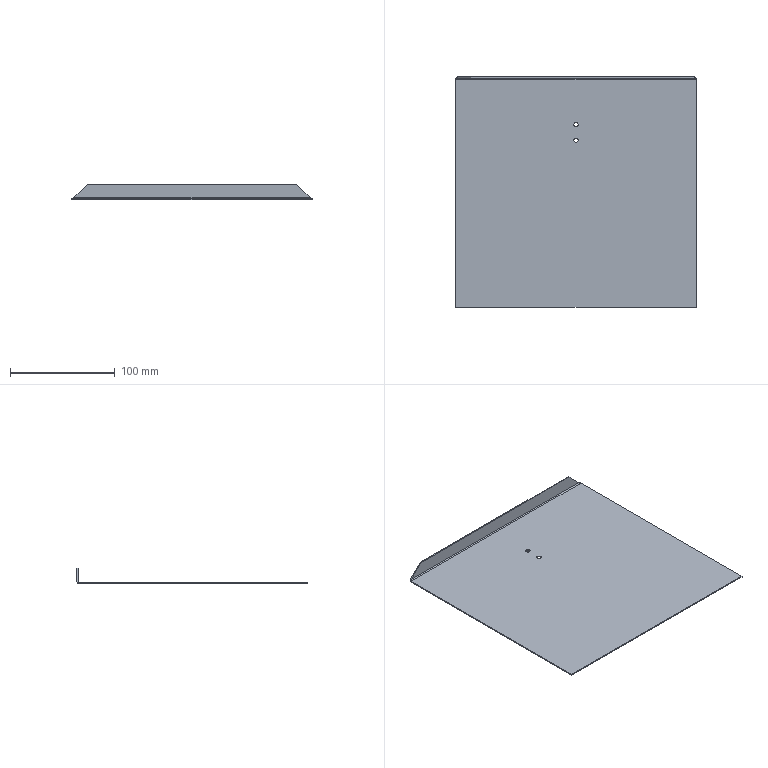Part | SolidWorks | features BaseBody 1 | 1 solid | 26 faces | box 230 x 220 x 15 mm | volume 53420 mm3 | plane 18 | cylinder 6 | spline 2 | commonest cylinder face diameters 4 x5 2 x1
STEP:
#1=CARTESIAN_POINT('',(113.,109.5,1.));
#2=VERTEX_POINT('',#1);
#3=CARTESIAN_POINT('',(113.,110.5,1.));
#4=VERTEX_POINT('',#3);
#5=CARTESIAN_POINT('',(113.,109.5,1.));
#6=DIRECTION('',(0.,1.,0.));
#7=VECTOR('',#6,1000.);
#8=LINE('',#5,#7);
#9=EDGE_CURVE('',#2,#4,#8,.T.);
#10=ORIENTED_EDGE('',*,*,#9,.F.);
#11=CARTESIAN_POINT('',(114.,108.5,0.));
#12=VERTEX_POINT('',#11);
#13=CARTESIAN_POINT('',(114.,108.5,0.));
#14=CARTESIAN_POINT('',(114.,109.086,0.));
#15=CARTESIAN_POINT('',(113.586,109.5,0.4142));
#16=CARTESIAN_POINT('',(113.,109.5,1.));
#17=(BOUNDED_CURVE()B_SPLINE_CURVE(3,(#13,#14,#15,#16),.UNSPECIFIED.,.F.,.F.)B_SPLINE_CURVE_WITH_KNOTS((4,4),(3.142,4.712),.UNSPECIFIED.)CURVE()GEOMETRIC_REPRESENTATION_ITEM()RATIONAL_B_SPLINE_CURVE((1.,0.8047,0.8047,1.))REPRESENTATION_ITEM(''));
#18=EDGE_CURVE('',#12,#2,#17,.T.);
#19=ORIENTED_EDGE('',*,*,#18,.F.);
#20=CARTESIAN_POINT('',(114.,108.5,-1.));
#21=VERTEX_POINT('',#20);
#22=CARTESIAN_POINT('',(114.,108.5,0.));
#23=DIRECTION('',(0.,0.,-1.));
#24=VECTOR('',#23,1000.);
#25=LINE('',#22,#24);
#26=EDGE_CURVE('',#12,#21,#25,.T.);
#27=ORIENTED_EDGE('',*,*,#26,.T.);
#28=CARTESIAN_POINT('',(114.,108.5,-1.));
#29=CARTESIAN_POINT('',(114.,109.672,-1.));
#30=CARTESIAN_POINT('',(113.586,110.5,-0.1716));
#31=CARTESIAN_POINT('',(113.,110.5,1.));
#32=(BOUNDED_CURVE()B_SPLINE_CURVE(3,(#28,#29,#30,#31),.UNSPECIFIED.,.F.,.F.)B_SPLINE_CURVE_WITH_KNOTS((4,4),(3.142,4.712),.UNSPECIFIED.)CURVE()GEOMETRIC_REPRESENTATION_ITEM()RATIONAL_B_SPLINE_CURVE((1.,0.8047,0.8047,1.))REPRESENTATION_ITEM(''));
#33=EDGE_CURVE('',#21,#4,#32,.T.);
#34=ORIENTED_EDGE('',*,*,#33,.T.);
#35=EDGE_LOOP('',(#10,#19,#27,#34));
#36=FACE_OUTER_BOUND('',#35,.T.);
#37=CARTESIAN_POINT('',(114.,108.5,-1.));
#38=CARTESIAN_POINT('',(114.,108.5,-0.6667));
#39=CARTESIAN_POINT('',(114.,108.5,-0.3333));
#40=CARTESIAN_POINT('',(114.,108.5,0.));
#41=CARTESIAN_POINT('',(114.,109.5,-1.));
#42=CARTESIAN_POINT('',(114.,109.333,-0.6667));
#43=CARTESIAN_POINT('',(114.,109.167,-0.3333));
#44=CARTESIAN_POINT('',(114.,109.,0.));
#45=CARTESIAN_POINT('',(113.667,110.5,-0.3333));
#46=CARTESIAN_POINT('',(113.667,110.167,-0.1111));
#47=CARTESIAN_POINT('',(113.667,109.833,0.1111));
#48=CARTESIAN_POINT('',(113.667,109.5,0.3333));
#49=CARTESIAN_POINT('',(113.,110.5,1.));
#50=CARTESIAN_POINT('',(113.,110.167,1.));
#51=CARTESIAN_POINT('',(113.,109.833,1.));
#52=CARTESIAN_POINT('',(113.,109.5,1.));
#53=(BOUNDED_SURFACE()B_SPLINE_SURFACE(3,3,((#37,#38,#39,#40),(#41,#42,#43,#44),(#45,#46,#47,#48),(#49,#50,#51,#52)),.UNSPECIFIED.,.F.,.F.,.T.)B_SPLINE_SURFACE_WITH_KNOTS((4,4),(4,4),(0.5,0.75),(0.,1.),.UNSPECIFIED.)GEOMETRIC_REPRESENTATION_ITEM()RATIONAL_B_SPLINE_SURFACE(((1.,1.,1.,1.),(0.6667,0.6667,0.6667,0.6667),(0.5,0.5,0.5,0.5),(0.5,0.5,0.5,0.5)))REPRESENTATION_ITEM('')SURFACE());
#54=ADVANCED_FACE('',(#36),#53,.T.);
#55=CARTESIAN_POINT('',(100.,109.5,14.));
#56=VERTEX_POINT('',#55);
#57=CARTESIAN_POINT('',(57.,109.5,57.));
#58=DIRECTION('',(0.7071,0.,-0.7071));
#59=VECTOR('',#58,1000.);
#60=LINE('',#57,#59);
#61=EDGE_CURVE('',#56,#2,#60,.T.);
#62=ORIENTED_EDGE('',*,*,#61,.T.);
#63=ORIENTED_EDGE('',*,*,#9,.T.);
#64=CARTESIAN_POINT('',(100.,110.5,14.));
#65=VERTEX_POINT('',#64);
#66=CARTESIAN_POINT('',(57.,110.5,57.));
#67=DIRECTION('',(0.7071,0.,-0.7071));
#68=VECTOR('',#67,1000.);
#69=LINE('',#66,#68);
#70=EDGE_CURVE('',#65,#4,#69,.T.);
#71=ORIENTED_EDGE('',*,*,#70,.F.);
#72=CARTESIAN_POINT('',(100.,109.5,14.));
#73=DIRECTION('',(0.,1.,0.));
#74=VECTOR('',#73,1000.);
#75=LINE('',#72,#74);
#76=EDGE_CURVE('',#56,#65,#75,.T.);
#77=ORIENTED_EDGE('',*,*,#76,.F.);
#78=EDGE_LOOP('',(#62,#63,#71,#77));
#79=FACE_OUTER_BOUND('',#78,.T.);
#80=CARTESIAN_POINT('',(57.,109.5,57.));
#81=DIRECTION('',(-0.7071,0.,-0.7071));
#82=DIRECTION('',(-0.7071,0.,0.7071));
#83=AXIS2_PLACEMENT_3D('',#80,#81,#82);
#84=PLANE('',#83);
#85=ADVANCED_FACE('',(#79),#84,.F.);
#86=CARTESIAN_POINT('',(-114.,108.5,0.));
#87=VERTEX_POINT('',#86);
#88=CARTESIAN_POINT('',(-114.,108.5,-1.));
#89=VERTEX_POINT('',#88);
#90=CARTESIAN_POINT('',(-114.,108.5,0.));
#91=DIRECTION('',(0.,0.,-1.));
#92=VECTOR('',#91,1000.);
#93=LINE('',#90,#92);
#94=EDGE_CURVE('',#87,#89,#93,.T.);
#95=ORIENTED_EDGE('',*,*,#94,.F.);
#96=CARTESIAN_POINT('',(-113.,109.5,1.));
#97=VERTEX_POINT('',#96);
#98=CARTESIAN_POINT('',(-113.,109.5,1.));
#99=CARTESIAN_POINT('',(-113.586,109.5,0.4142));
#100=CARTESIAN_POINT('',(-114.,109.086,0.));
#101=CARTESIAN_POINT('',(-114.,108.5,0.));
#102=(BOUNDED_CURVE()B_SPLINE_CURVE(3,(#98,#99,#100,#101),.UNSPECIFIED.,.F.,.F.)B_SPLINE_CURVE_WITH_KNOTS((4,4),(4.712,6.283),.UNSPECIFIED.)CURVE()GEOMETRIC_REPRESENTATION_ITEM()RATIONAL_B_SPLINE_CURVE((1.,0.8047,0.8047,1.))REPRESENTATION_ITEM(''));
#103=EDGE_CURVE('',#97,#87,#102,.T.);
#104=ORIENTED_EDGE('',*,*,#103,.F.);
#105=CARTESIAN_POINT('',(-113.,110.5,1.));
#106=VERTEX_POINT('',#105);
#107=CARTESIAN_POINT('',(-113.,110.5,1.));
#108=DIRECTION('',(0.,-1.,0.));
#109=VECTOR('',#108,1000.);
#110=LINE('',#107,#109);
#111=EDGE_CURVE('',#106,#97,#110,.T.);
#112=ORIENTED_EDGE('',*,*,#111,.F.);
#113=CARTESIAN_POINT('',(-113.,110.5,1.));
#114=CARTESIAN_POINT('',(-113.586,110.5,-0.1716));
#115=CARTESIAN_POINT('',(-114.,109.672,-1.));
#116=CARTESIAN_POINT('',(-114.,108.5,-1.));
#117=(BOUNDED_CURVE()B_SPLINE_CURVE(3,(#113,#114,#115,#116),.UNSPECIFIED.,.F.,.F.)B_SPLINE_CURVE_WITH_KNOTS((4,4),(4.712,6.283),.UNSPECIFIED.)CURVE()GEOMETRIC_REPRESENTATION_ITEM()RATIONAL_B_SPLINE_CURVE((1.,0.8047,0.8047,1.))REPRESENTATION_ITEM(''));
#118=EDGE_CURVE('',#106,#89,#117,.T.);
#119=ORIENTED_EDGE('',*,*,#118,.T.);
#120=EDGE_LOOP('',(#95,#104,#112,#119));
#121=FACE_OUTER_BOUND('',#120,.T.);
#122=CARTESIAN_POINT('',(-113.,110.5,1.));
#123=CARTESIAN_POINT('',(-113.,110.167,1.));
#124=CARTESIAN_POINT('',(-113.,109.833,1.));
#125=CARTESIAN_POINT('',(-113.,109.5,1.));
#126=CARTESIAN_POINT('',(-113.667,110.5,-0.3333));
#127=CARTESIAN_POINT('',(-113.667,110.167,-0.1111));
#128=CARTESIAN_POINT('',(-113.667,109.833,0.1111));
#129=CARTESIAN_POINT('',(-113.667,109.5,0.3333));
#130=CARTESIAN_POINT('',(-114.,109.5,-1.));
#131=CARTESIAN_POINT('',(-114.,109.333,-0.6667));
#132=CARTESIAN_POINT('',(-114.,109.167,-0.3333));
#133=CARTESIAN_POINT('',(-114.,109.,0.));
#134=CARTESIAN_POINT('',(-114.,108.5,-1.));
#135=CARTESIAN_POINT('',(-114.,108.5,-0.6667));
#136=CARTESIAN_POINT('',(-114.,108.5,-0.3333));
#137=CARTESIAN_POINT('',(-114.,108.5,0.));
#138=(BOUNDED_SURFACE()B_SPLINE_SURFACE(3,3,((#122,#123,#124,#125),(#126,#127,#128,#129),(#130,#131,#132,#133),(#134,#135,#136,#137)),.UNSPECIFIED.,.F.,.F.,.T.)B_SPLINE_SURFACE_WITH_KNOTS((4,4),(4,4),(0.75,1.),(0.,1.),.UNSPECIFIED.)GEOMETRIC_REPRESENTATION_ITEM()RATIONAL_B_SPLINE_SURFACE(((0.5,0.5,0.5,0.5),(0.5,0.5,0.5,0.5),(0.6667,0.6667,0.6667,0.6667),(1.,1.,1.,1.)))REPRESENTATION_ITEM('')SURFACE());
#139=ADVANCED_FACE('',(#121),#138,.T.);
#140=CARTESIAN_POINT('',(-100.,110.5,14.));
#141=VERTEX_POINT('',#140);
#142=CARTESIAN_POINT('',(-100.,109.5,14.));
#143=VERTEX_POINT('',#142);
#144=CARTESIAN_POINT('',(-100.,110.5,14.));
#145=DIRECTION('',(0.,-1.,0.));
#146=VECTOR('',#145,1000.);
#147=LINE('',#144,#146);
#148=EDGE_CURVE('',#141,#143,#147,.T.);
#149=ORIENTED_EDGE('',*,*,#148,.F.);
#150=CARTESIAN_POINT('',(-114.,110.5,0.));
#151=DIRECTION('',(-0.7071,0.,-0.7071));
#152=VECTOR('',#151,1000.);
#153=LINE('',#150,#152);
#154=EDGE_CURVE('',#141,#106,#153,.T.);
#155=ORIENTED_EDGE('',*,*,#154,.T.);
#156=ORIENTED_EDGE('',*,*,#111,.T.);
#157=CARTESIAN_POINT('',(-114.,109.5,0.));
#158=DIRECTION('',(-0.7071,0.,-0.7071));
#159=VECTOR('',#158,1000.);
#160=LINE('',#157,#159);
#161=EDGE_CURVE('',#143,#97,#160,.T.);
#162=ORIENTED_EDGE('',*,*,#161,.F.);
#163=EDGE_LOOP('',(#149,#155,#156,#162));
#164=FACE_OUTER_BOUND('',#163,.T.);
#165=CARTESIAN_POINT('',(-114.,110.5,0.));
#166=DIRECTION('',(-0.7071,0.,0.7071));
#167=DIRECTION('',(0.,1.,0.));
#168=AXIS2_PLACEMENT_3D('',#165,#166,#167);
#169=PLANE('',#168);
#170=ADVANCED_FACE('',(#164),#169,.T.);
#171=CARTESIAN_POINT('',(114.5,109.5,0.));
#172=VERTEX_POINT('',#171);
#173=CARTESIAN_POINT('',(114.5,109.5,-1.));
#174=VERTEX_POINT('',#173);
#175=CARTESIAN_POINT('',(114.5,109.5,0.));
#176=DIRECTION('',(0.,0.,-1.));
#177=VECTOR('',#176,1000.);
#178=LINE('',#175,#177);
#179=EDGE_CURVE('',#172,#174,#178,.T.);
#180=ORIENTED_EDGE('',*,*,#179,.T.);
#181=CARTESIAN_POINT('',(114.5,108.,-1.));
#182=VERTEX_POINT('',#181);
#183=CARTESIAN_POINT('',(114.5,-109.5,-1.));
#184=DIRECTION('',(0.,-1.,0.));
#185=VECTOR('',#184,1000.);
#186=LINE('',#183,#185);
#187=EDGE_CURVE('',#174,#182,#186,.T.);
#188=ORIENTED_EDGE('',*,*,#187,.T.);
#189=CARTESIAN_POINT('',(114.5,108.,0.));
#190=VERTEX_POINT('',#189);
#191=CARTESIAN_POINT('',(114.5,108.,0.));
#192=DIRECTION('',(0.,0.,-1.));
#193=VECTOR('',#192,1000.);
#194=LINE('',#191,#193);
#195=EDGE_CURVE('',#190,#182,#194,.T.);
#196=ORIENTED_EDGE('',*,*,#195,.F.);
#197=CARTESIAN_POINT('',(114.5,108.,0.));
#198=DIRECTION('',(0.,1.,0.));
#199=VECTOR('',#198,1000.);
#200=LINE('',#197,#199);
#201=EDGE_CURVE('',#190,#172,#200,.T.);
#202=ORIENTED_EDGE('',*,*,#201,.T.);
#203=EDGE_LOOP('',(#180,#188,#196,#202));
#204=FACE_OUTER_BOUND('',#203,.T.);
#205=CARTESIAN_POINT('',(114.5,108.,0.));
#206=DIRECTION('',(-1.,0.,0.));
#207=DIRECTION('',(0.,1.,0.));
#208=AXIS2_PLACEMENT_3D('',#205,#206,#207);
#209=PLANE('',#208);
#210=ADVANCED_FACE('',(#204),#209,.T.);
#211=ORIENTED_EDGE('',*,*,#195,.T.);
#212=CARTESIAN_POINT('',(114.,108.,-1.));
#213=VERTEX_POINT('',#212);
#214=CARTESIAN_POINT('',(115.,108.,-1.));
#215=DIRECTION('',(-1.,0.,0.));
#216=VECTOR('',#215,1000.);
#217=LINE('',#214,#216);
#218=EDGE_CURVE('',#182,#213,#217,.T.);
#219=ORIENTED_EDGE('',*,*,#218,.T.);
#220=CARTESIAN_POINT('',(114.,108.,0.));
#221=VERTEX_POINT('',#220);
#222=CARTESIAN_POINT('',(114.,108.,0.));
#223=DIRECTION('',(0.,0.,-1.));
#224=VECTOR('',#223,1000.);
#225=LINE('',#222,#224);
#226=EDGE_CURVE('',#221,#213,#225,.T.);
#227=ORIENTED_EDGE('',*,*,#226,.F.);
#228=CARTESIAN_POINT('',(114.,108.,0.));
#229=DIRECTION('',(1.,0.,0.));
#230=VECTOR('',#229,1000.);
#231=LINE('',#228,#230);
#232=EDGE_CURVE('',#221,#190,#231,.T.);
#233=ORIENTED_EDGE('',*,*,#232,.T.);
#234=EDGE_LOOP('',(#211,#219,#227,#233));
#235=FACE_OUTER_BOUND('',#234,.T.);
#236=CARTESIAN_POINT('',(114.,108.,0.));
#237=DIRECTION('',(0.,1.,0.));
#238=DIRECTION('',(0.,0.,-1.));
#239=AXIS2_PLACEMENT_3D('',#236,#237,#238);
#240=PLANE('',#239);
#241=ADVANCED_FACE('',(#235),#240,.T.);
#242=ORIENTED_EDGE('',*,*,#226,.T.);
#243=CARTESIAN_POINT('',(114.,-109.5,-1.));
#244=DIRECTION('',(0.,1.,0.));
#245=VECTOR('',#244,1000.);
#246=LINE('',#243,#245);
#247=EDGE_CURVE('',#213,#21,#246,.T.);
#248=ORIENTED_EDGE('',*,*,#247,.T.);
#249=ORIENTED_EDGE('',*,*,#26,.F.);
#250=CARTESIAN_POINT('',(114.,108.5,0.));
#251=DIRECTION('',(0.,-1.,0.));
#252=VECTOR('',#251,1000.);
#253=LINE('',#250,#252);
#254=EDGE_CURVE('',#12,#221,#253,.T.);
#255=ORIENTED_EDGE('',*,*,#254,.T.);
#256=EDGE_LOOP('',(#242,#248,#249,#255));
#257=FACE_OUTER_BOUND('',#256,.T.);
#258=CARTESIAN_POINT('',(114.,108.5,0.));
#259=DIRECTION('',(1.,0.,0.));
#260=DIRECTION('',(0.,1.,0.));
#261=AXIS2_PLACEMENT_3D('',#258,#259,#260);
#262=PLANE('',#261);
#263=ADVANCED_FACE('',(#257),#262,.T.);
#264=ORIENTED_EDGE('',*,*,#94,.T.);
#265=CARTESIAN_POINT('',(-114.,108.,-1.));
#266=VERTEX_POINT('',#265);
#267=CARTESIAN_POINT('',(-114.,-109.5,-1.));
#268=DIRECTION('',(0.,-1.,0.));
#269=VECTOR('',#268,1000.);
#270=LINE('',#267,#269);
#271=EDGE_CURVE('',#89,#266,#270,.T.);
#272=ORIENTED_EDGE('',*,*,#271,.T.);
#273=CARTESIAN_POINT('',(-114.,108.,0.));
#274=VERTEX_POINT('',#273);
#275=CARTESIAN_POINT('',(-114.,108.,0.));
#276=DIRECTION('',(0.,0.,-1.));
#277=VECTOR('',#276,1000.);
#278=LINE('',#275,#277);
#279=EDGE_CURVE('',#274,#266,#278,.T.);
#280=ORIENTED_EDGE('',*,*,#279,.F.);
#281=CARTESIAN_POINT('',(-114.,108.,0.));
#282=DIRECTION('',(0.,1.,0.));
#283=VECTOR('',#282,1000.);
#284=LINE('',#281,#283);
#285=EDGE_CURVE('',#274,#87,#284,.T.);
#286=ORIENTED_EDGE('',*,*,#285,.T.);
#287=EDGE_LOOP('',(#264,#272,#280,#286));
#288=FACE_OUTER_BOUND('',#287,.T.);
#289=CARTESIAN_POINT('',(-114.,108.,0.));
#290=DIRECTION('',(-1.,0.,0.));
#291=DIRECTION('',(0.,0.,1.));
#292=AXIS2_PLACEMENT_3D('',#289,#290,#291);
#293=PLANE('',#292);
#294=ADVANCED_FACE('',(#288),#293,.T.);
#295=ORIENTED_EDGE('',*,*,#279,.T.);
#296=CARTESIAN_POINT('',(-114.5,108.,-1.));
#297=VERTEX_POINT('',#296);
#298=CARTESIAN_POINT('',(115.,108.,-1.));
#299=DIRECTION('',(-1.,0.,0.));
#300=VECTOR('',#299,1000.);
#301=LINE('',#298,#300);
#302=EDGE_CURVE('',#266,#297,#301,.T.);
#303=ORIENTED_EDGE('',*,*,#302,.T.);
#304=CARTESIAN_POINT('',(-114.5,108.,0.));
#305=VERTEX_POINT('',#304);
#306=CARTESIAN_POINT('',(-114.5,108.,0.));
#307=DIRECTION('',(0.,0.,-1.));
#308=VECTOR('',#307,1000.);
#309=LINE('',#306,#308);
#310=EDGE_CURVE('',#305,#297,#309,.T.);
#311=ORIENTED_EDGE('',*,*,#310,.F.);
#312=CARTESIAN_POINT('',(-114.5,108.,0.));
#313=DIRECTION('',(1.,0.,0.));
#314=VECTOR('',#313,1000.);
#315=LINE('',#312,#314);
#316=EDGE_CURVE('',#305,#274,#315,.T.);
#317=ORIENTED_EDGE('',*,*,#316,.T.);
#318=EDGE_LOOP('',(#295,#303,#311,#317));
#319=FACE_OUTER_BOUND('',#318,.T.);
#320=CARTESIAN_POINT('',(-114.5,108.,0.));
#321=DIRECTION('',(0.,1.,0.));
#322=DIRECTION('',(0.,0.,-1.));
#323=AXIS2_PLACEMENT_3D('',#320,#321,#322);
#324=PLANE('',#323);
#325=ADVANCED_FACE('',(#319),#324,.T.);
#326=ORIENTED_EDGE('',*,*,#310,.T.);
#327=CARTESIAN_POINT('',(-114.5,109.5,-1.));
#328=VERTEX_POINT('',#327);
#329=CARTESIAN_POINT('',(-114.5,-109.5,-1.));
#330=DIRECTION('',(0.,1.,0.));
#331=VECTOR('',#330,1000.);
#332=LINE('',#329,#331);
#333=EDGE_CURVE('',#297,#328,#332,.T.);
#334=ORIENTED_EDGE('',*,*,#333,.T.);
#335=CARTESIAN_POINT('',(-114.5,109.5,0.));
#336=VERTEX_POINT('',#335);
#337=CARTESIAN_POINT('',(-114.5,109.5,0.));
#338=DIRECTION('',(0.,0.,-1.));
#339=VECTOR('',#338,1000.);
#340=LINE('',#337,#339);
#341=EDGE_CURVE('',#336,#328,#340,.T.);
#342=ORIENTED_EDGE('',*,*,#341,.F.);
#343=CARTESIAN_POINT('',(-114.5,109.5,0.));
#344=DIRECTION('',(0.,-1.,0.));
#345=VECTOR('',#344,1000.);
#346=LINE('',#343,#345);
#347=EDGE_CURVE('',#336,#305,#346,.T.);
#348=ORIENTED_EDGE('',*,*,#347,.T.);
#349=EDGE_LOOP('',(#326,#334,#342,#348));
#350=FACE_OUTER_BOUND('',#349,.T.);
#351=CARTESIAN_POINT('',(-114.5,109.5,0.));
#352=DIRECTION('',(1.,0.,0.));
#353=DIRECTION('',(0.,1.,0.));
#354=AXIS2_PLACEMENT_3D('',#351,#352,#353);
#355=PLANE('',#354);
#356=ADVANCED_FACE('',(#350),#355,.T.);
#357=CARTESIAN_POINT('',(2.,65.,0.));
#358=VERTEX_POINT('',#357);
#359=CARTESIAN_POINT('',(2.,65.,-1.));
#360=VERTEX_POINT('',#359);
#361=CARTESIAN_POINT('',(2.,65.,9.));
#362=DIRECTION('',(0.,0.,-1.));
#363=VECTOR('',#362,1000.);
#364=LINE('',#361,#363);
#365=EDGE_CURVE('',#358,#360,#364,.T.);
#366=ORIENTED_EDGE('',*,*,#365,.F.);
#367=CARTESIAN_POINT('',(-2.,65.,0.));
#368=VERTEX_POINT('',#367);
#369=CARTESIAN_POINT('',(0.,65.,0.));
#370=DIRECTION('',(0.,0.,1.));
#371=DIRECTION('',(1.,0.,0.));
#372=AXIS2_PLACEMENT_3D('',#369,#370,#371);
#373=CIRCLE('',#372,2.);
#374=EDGE_CURVE('',#358,#368,#373,.T.);
#375=ORIENTED_EDGE('',*,*,#374,.T.);
#376=CARTESIAN_POINT('',(-2.,65.,-1.));
#377=VERTEX_POINT('',#376);
#378=CARTESIAN_POINT('',(-2.,65.,9.));
#379=DIRECTION('',(0.,0.,-1.));
#380=VECTOR('',#379,1000.);
#381=LINE('',#378,#380);
#382=EDGE_CURVE('',#368,#377,#381,.T.);
#383=ORIENTED_EDGE('',*,*,#382,.T.);
#384=CARTESIAN_POINT('',(0.,65.,-1.));
#385=DIRECTION('',(0.,0.,-1.));
#386=DIRECTION('',(-1.,0.,0.));
#387=AXIS2_PLACEMENT_3D('',#384,#385,#386);
#388=CIRCLE('',#387,2.);
#389=EDGE_CURVE('',#377,#360,#388,.T.);
#390=ORIENTED_EDGE('',*,*,#389,.T.);
#391=EDGE_LOOP('',(#366,#375,#383,#390));
#392=FACE_OUTER_BOUND('',#391,.T.);
#393=CARTESIAN_POINT('',(0.,65.,9.));
#394=DIRECTION('',(0.,0.,-1.));
#395=DIRECTION('',(-1.,0.,0.));
#396=AXIS2_PLACEMENT_3D('',#393,#394,#395);
#397=CYLINDRICAL_SURFACE('',#396,2.);
#398=ADVANCED_FACE('',(#392),#397,.F.);
#399=CARTESIAN_POINT('',(2.,50.,0.));
#400=VERTEX_POINT('',#399);
#401=CARTESIAN_POINT('',(2.,50.,-1.));
#402=VERTEX_POINT('',#401);
#403=CARTESIAN_POINT('',(2.,50.,9.));
#404=DIRECTION('',(0.,0.,-1.));
#405=VECTOR('',#404,1000.);
#406=LINE('',#403,#405);
#407=EDGE_CURVE('',#400,#402,#406,.T.);
#408=ORIENTED_EDGE('',*,*,#407,.F.);
#409=CARTESIAN_POINT('',(-2.,50.,0.));
#410=VERTEX_POINT('',#409);
#411=CARTESIAN_POINT('',(0.,50.,0.));
#412=DIRECTION('',(0.,0.,1.));
#413=DIRECTION('',(1.,0.,0.));
#414=AXIS2_PLACEMENT_3D('',#411,#412,#413);
#415=CIRCLE('',#414,2.);
#416=EDGE_CURVE('',#400,#410,#415,.T.);
#417=ORIENTED_EDGE('',*,*,#416,.T.);
#418=CARTESIAN_POINT('',(-2.,50.,-1.));
#419=VERTEX_POINT('',#418);
#420=CARTESIAN_POINT('',(-2.,50.,9.));
#421=DIRECTION('',(0.,0.,-1.));
#422=VECTOR('',#421,1000.);
#423=LINE('',#420,#422);
#424=EDGE_CURVE('',#410,#419,#423,.T.);
#425=ORIENTED_EDGE('',*,*,#424,.T.);
#426=CARTESIAN_POINT('',(0.,50.,-1.));
#427=DIRECTION('',(0.,0.,-1.));
#428=DIRECTION('',(-1.,0.,0.));
#429=AXIS2_PLACEMENT_3D('',#426,#427,#428);
#430=CIRCLE('',#429,2.);
#431=EDGE_CURVE('',#419,#402,#430,.T.);
#432=ORIENTED_EDGE('',*,*,#431,.T.);
#433=EDGE_LOOP('',(#408,#417,#425,#432));
#434=FACE_OUTER_BOUND('',#433,.T.);
#435=CARTESIAN_POINT('',(0.,50.,9.));
#436=DIRECTION('',(0.,0.,-1.));
#437=DIRECTION('',(-1.,0.,0.));
#438=AXIS2_PLACEMENT_3D('',#435,#436,#437);
#439=CYLINDRICAL_SURFACE('',#438,2.);
#440=ADVANCED_FACE('',(#434),#439,.F.);
#441=CARTESIAN_POINT('',(-115.,109.5,0.));
#442=VERTEX_POINT('',#441);
#443=CARTESIAN_POINT('',(-115.,-109.5,0.));
#444=VERTEX_POINT('',#443);
#445=CARTESIAN_POINT('',(-115.,109.5,0.));
#446=DIRECTION('',(0.,-1.,0.));
#447=VECTOR('',#446,1000.);
#448=LINE('',#445,#447);
#449=EDGE_CURVE('',#442,#444,#448,.T.);
#450=ORIENTED_EDGE('',*,*,#449,.F.);
#451=CARTESIAN_POINT('',(-115.,109.5,-1.));
#452=VERTEX_POINT('',#451);
#453=CARTESIAN_POINT('',(-115.,109.5,-1.));
#454=DIRECTION('',(0.,0.,1.));
#455=VECTOR('',#454,1000.);
#456=LINE('',#453,#455);
#457=EDGE_CURVE('',#452,#442,#456,.T.);
#458=ORIENTED_EDGE('',*,*,#457,.F.);
#459=CARTESIAN_POINT('',(-115.,-109.5,-1.));
#460=VERTEX_POINT('',#459);
#461=CARTESIAN_POINT('',(-115.,109.5,-1.));
#462=DIRECTION('',(0.,-1.,0.));
#463=VECTOR('',#462,1000.);
#464=LINE('',#461,#463);
#465=EDGE_CURVE('',#452,#460,#464,.T.);
#466=ORIENTED_EDGE('',*,*,#465,.T.);
#467=CARTESIAN_POINT('',(-115.,-109.5,-1.));
#468=DIRECTION('',(0.,0.,1.));
#469=VECTOR('',#468,1000.);
#470=LINE('',#467,#469);
#471=EDGE_CURVE('',#460,#444,#470,.T.);
#472=ORIENTED_EDGE('',*,*,#471,.T.);
#473=EDGE_LOOP('',(#450,#458,#466,#472));
#474=FACE_OUTER_BOUND('',#473,.T.);
#475=CARTESIAN_POINT('',(-115.,109.5,-1.));
#476=DIRECTION('',(-1.,0.,0.));
#477=DIRECTION('',(0.,1.,0.));
#478=AXIS2_PLACEMENT_3D('',#475,#476,#477);
#479=PLANE('',#478);
#480=ADVANCED_FACE('',(#474),#479,.T.);
#481=CARTESIAN_POINT('',(115.,-109.5,0.));
#482=VERTEX_POINT('',#481);
#483=CARTESIAN_POINT('',(-115.,-109.5,0.));
#484=DIRECTION('',(1.,0.,0.));
#485=VECTOR('',#484,1000.);
#486=LINE('',#483,#485);
#487=EDGE_CURVE('',#444,#482,#486,.T.);
#488=ORIENTED_EDGE('',*,*,#487,.F.);
#489=ORIENTED_EDGE('',*,*,#471,.F.);
#490=CARTESIAN_POINT('',(115.,-109.5,-1.));
#491=VERTEX_POINT('',#490);
#492=CARTESIAN_POINT('',(-115.,-109.5,-1.));
#493=DIRECTION('',(1.,0.,0.));
#494=VECTOR('',#493,1000.);
#495=LINE('',#492,#494);
#496=EDGE_CURVE('',#460,#491,#495,.T.);
#497=ORIENTED_EDGE('',*,*,#496,.T.);
#498=CARTESIAN_POINT('',(115.,-109.5,-1.));
#499=DIRECTION('',(0.,0.,1.));
#500=VECTOR('',#499,1000.);
#501=LINE('',#498,#500);
#502=EDGE_CURVE('',#491,#482,#501,.T.);
#503=ORIENTED_EDGE('',*,*,#502,.T.);
#504=EDGE_LOOP('',(#488,#489,#497,#503));
#505=FACE_OUTER_BOUND('',#504,.T.);
#506=CARTESIAN_POINT('',(-115.,-109.5,-1.));
#507=DIRECTION('',(0.,-1.,0.));
#508=DIRECTION('',(0.,0.,-1.));
#509=AXIS2_PLACEMENT_3D('',#506,#507,#508);
#510=PLANE('',#509);
#511=ADVANCED_FACE('',(#505),#510,.T.);
#512=CARTESIAN_POINT('',(115.,109.5,0.));
#513=VERTEX_POINT('',#512);
#514=CARTESIAN_POINT('',(115.,109.5,0.));
#515=DIRECTION('',(0.,1.,0.));
#516=VECTOR('',#515,1000.);
#517=LINE('',#514,#516);
#518=EDGE_CURVE('',#482,#513,#517,.T.);
#519=ORIENTED_EDGE('',*,*,#518,.F.);
#520=ORIENTED_EDGE('',*,*,#502,.F.);
#521=CARTESIAN_POINT('',(115.,109.5,-1.));
#522=VERTEX_POINT('',#521);
#523=CARTESIAN_POINT('',(115.,109.5,-1.));
#524=DIRECTION('',(0.,1.,0.));
#525=VECTOR('',#524,1000.);
#526=LINE('',#523,#525);
#527=EDGE_CURVE('',#491,#522,#526,.T.);
#528=ORIENTED_EDGE('',*,*,#527,.T.);
#529=CARTESIAN_POINT('',(115.,109.5,-1.));
#530=DIRECTION('',(0.,0.,1.));
#531=VECTOR('',#530,1000.);
#532=LINE('',#529,#531);
#533=EDGE_CURVE('',#522,#513,#532,.T.);
#534=ORIENTED_EDGE('',*,*,#533,.T.);
#535=EDGE_LOOP('',(#519,#520,#528,#534));
#536=FACE_OUTER_BOUND('',#535,.T.);
#537=CARTESIAN_POINT('',(115.,109.5,-1.));
#538=DIRECTION('',(1.,0.,0.));
#539=DIRECTION('',(0.,1.,0.));
#540=AXIS2_PLACEMENT_3D('',#537,#538,#539);
#541=PLANE('',#540);
#542=ADVANCED_FACE('',(#536),#541,.T.);
#543=CARTESIAN_POINT('',(0.,50.,0.));
#544=DIRECTION('',(0.,0.,1.));
#545=DIRECTION('',(1.,0.,0.));
#546=AXIS2_PLACEMENT_3D('',#543,#544,#545);
#547=CIRCLE('',#546,2.);
#548=EDGE_CURVE('',#410,#400,#547,.T.);
#549=ORIENTED_EDGE('',*,*,#548,.F.);
#550=ORIENTED_EDGE('',*,*,#416,.F.);
#551=EDGE_LOOP('',(#549,#550));
#552=FACE_BOUND('',#551,.T.);
#553=CARTESIAN_POINT('',(0.,65.,0.));
#554=DIRECTION('',(0.,0.,1.));
#555=DIRECTION('',(1.,0.,0.));
#556=AXIS2_PLACEMENT_3D('',#553,#554,#555);
#557=CIRCLE('',#556,2.);
#558=EDGE_CURVE('',#368,#358,#557,.T.);
#559=ORIENTED_EDGE('',*,*,#558,.F.);
#560=ORIENTED_EDGE('',*,*,#374,.F.);
#561=EDGE_LOOP('',(#559,#560));
#562=FACE_BOUND('',#561,.T.);
#563=ORIENTED_EDGE('',*,*,#316,.F.);
#564=ORIENTED_EDGE('',*,*,#347,.F.);
#565=CARTESIAN_POINT('',(-115.,109.5,0.));
#566=DIRECTION('',(-1.,0.,0.));
#567=VECTOR('',#566,1000.);
#568=LINE('',#565,#567);
#569=EDGE_CURVE('',#336,#442,#568,.T.);
#570=ORIENTED_EDGE('',*,*,#569,.T.);
#571=ORIENTED_EDGE('',*,*,#449,.T.);
#572=ORIENTED_EDGE('',*,*,#487,.T.);
#573=ORIENTED_EDGE('',*,*,#518,.T.);
#574=CARTESIAN_POINT('',(-115.,109.5,0.));
#575=DIRECTION('',(-1.,0.,0.));
#576=VECTOR('',#575,1000.);
#577=LINE('',#574,#576);
#578=EDGE_CURVE('',#513,#172,#577,.T.);
#579=ORIENTED_EDGE('',*,*,#578,.T.);
#580=ORIENTED_EDGE('',*,*,#201,.F.);
#581=ORIENTED_EDGE('',*,*,#232,.F.);
#582=ORIENTED_EDGE('',*,*,#254,.F.);
#583=CARTESIAN_POINT('',(-114.,108.5,0.));
#584=DIRECTION('',(1.,0.,0.));
#585=VECTOR('',#584,1000.);
#586=LINE('',#583,#585);
#587=EDGE_CURVE('',#87,#12,#586,.T.);
#588=ORIENTED_EDGE('',*,*,#587,.F.);
#589=ORIENTED_EDGE('',*,*,#285,.F.);
#590=EDGE_LOOP('',(#563,#564,#570,#571,#572,#573,#579,#580,#581,#582,#588,#589));
#591=FACE_OUTER_BOUND('',#590,.T.);
#592=CARTESIAN_POINT('',(115.,-109.5,0.));
#593=DIRECTION('',(0.,0.,1.));
#594=DIRECTION('',(1.,0.,0.));
#595=AXIS2_PLACEMENT_3D('',#592,#593,#594);
#596=PLANE('',#595);
#597=ADVANCED_FACE('',(#552,#562,#591),#596,.T.);
#598=ORIENTED_EDGE('',*,*,#389,.F.);
#599=CARTESIAN_POINT('',(0.,65.,-1.));
#600=DIRECTION('',(0.,0.,-1.));
#601=DIRECTION('',(-1.,0.,0.));
#602=AXIS2_PLACEMENT_3D('',#599,#600,#601);
#603=CIRCLE('',#602,2.);
#604=EDGE_CURVE('',#360,#377,#603,.T.);
#605=ORIENTED_EDGE('',*,*,#604,.F.);
#606=EDGE_LOOP('',(#598,#605));
#607=FACE_BOUND('',#606,.T.);
#608=ORIENTED_EDGE('',*,*,#431,.F.);
#609=CARTESIAN_POINT('',(0.,50.,-1.));
#610=DIRECTION('',(0.,0.,-1.));
#611=DIRECTION('',(-1.,0.,0.));
#612=AXIS2_PLACEMENT_3D('',#609,#610,#611);
#613=CIRCLE('',#612,2.);
#614=EDGE_CURVE('',#402,#419,#613,.T.);
#615=ORIENTED_EDGE('',*,*,#614,.F.);
#616=EDGE_LOOP('',(#608,#615));
#617=FACE_BOUND('',#616,.T.);
#618=ORIENTED_EDGE('',*,*,#333,.F.);
#619=ORIENTED_EDGE('',*,*,#302,.F.);
#620=ORIENTED_EDGE('',*,*,#271,.F.);
#621=CARTESIAN_POINT('',(-114.,108.5,-1.));
#622=DIRECTION('',(1.,0.,0.));
#623=VECTOR('',#622,1000.);
#624=LINE('',#621,#623);
#625=EDGE_CURVE('',#89,#21,#624,.T.);
#626=ORIENTED_EDGE('',*,*,#625,.T.);
#627=ORIENTED_EDGE('',*,*,#247,.F.);
#628=ORIENTED_EDGE('',*,*,#218,.F.);
#629=ORIENTED_EDGE('',*,*,#187,.F.);
#630=CARTESIAN_POINT('',(-115.,109.5,-1.));
#631=DIRECTION('',(-1.,0.,0.));
#632=VECTOR('',#631,1000.);
#633=LINE('',#630,#632);
#634=EDGE_CURVE('',#522,#174,#633,.T.);
#635=ORIENTED_EDGE('',*,*,#634,.F.);
#636=ORIENTED_EDGE('',*,*,#527,.F.);
#637=ORIENTED_EDGE('',*,*,#496,.F.);
#638=ORIENTED_EDGE('',*,*,#465,.F.);
#639=CARTESIAN_POINT('',(-115.,109.5,-1.));
#640=DIRECTION('',(-1.,0.,0.));
#641=VECTOR('',#640,1000.);
#642=LINE('',#639,#641);
#643=EDGE_CURVE('',#328,#452,#642,.T.);
#644=ORIENTED_EDGE('',*,*,#643,.F.);
#645=EDGE_LOOP('',(#618,#619,#620,#626,#627,#628,#629,#635,#636,#637,#638,#644));
#646=FACE_OUTER_BOUND('',#645,.T.);
#647=CARTESIAN_POINT('',(115.,-109.5,-1.));
#648=DIRECTION('',(0.,0.,1.));
#649=DIRECTION('',(1.,0.,0.));
#650=AXIS2_PLACEMENT_3D('',#647,#648,#649);
#651=PLANE('',#650);
#652=ADVANCED_FACE('',(#607,#617,#646),#651,.F.);
#653=ORIENTED_EDGE('',*,*,#634,.T.);
#654=ORIENTED_EDGE('',*,*,#179,.F.);
#655=ORIENTED_EDGE('',*,*,#578,.F.);
#656=ORIENTED_EDGE('',*,*,#533,.F.);
#657=EDGE_LOOP('',(#653,#654,#655,#656));
#658=FACE_OUTER_BOUND('',#657,.T.);
#659=CARTESIAN_POINT('',(-115.,109.5,-1.));
#660=DIRECTION('',(0.,1.,0.));
#661=DIRECTION('',(1.,0.,0.));
#662=AXIS2_PLACEMENT_3D('',#659,#660,#661);
#663=PLANE('',#662);
#664=ADVANCED_FACE('',(#658),#663,.T.);
#665=ORIENTED_EDGE('',*,*,#569,.F.);
#666=ORIENTED_EDGE('',*,*,#341,.T.);
#667=ORIENTED_EDGE('',*,*,#643,.T.);
#668=ORIENTED_EDGE('',*,*,#457,.T.);
#669=EDGE_LOOP('',(#665,#666,#667,#668));
#670=FACE_OUTER_BOUND('',#669,.T.);
#671=CARTESIAN_POINT('',(-115.,109.5,-1.));
#672=DIRECTION('',(0.,1.,0.));
#673=DIRECTION('',(1.,0.,0.));
#674=AXIS2_PLACEMENT_3D('',#671,#672,#673);
#675=PLANE('',#674);
#676=ADVANCED_FACE('',(#670),#675,.T.);
#677=ORIENTED_EDGE('',*,*,#76,.T.);
#678=CARTESIAN_POINT('',(114.,110.5,14.));
#679=DIRECTION('',(1.,0.,0.));
#680=VECTOR('',#679,1000.);
#681=LINE('',#678,#680);
#682=EDGE_CURVE('',#141,#65,#681,.T.);
#683=ORIENTED_EDGE('',*,*,#682,.F.);
#684=ORIENTED_EDGE('',*,*,#148,.T.);
#685=CARTESIAN_POINT('',(114.,109.5,14.));
#686=DIRECTION('',(1.,0.,0.));
#687=VECTOR('',#686,1000.);
#688=LINE('',#685,#687);
#689=EDGE_CURVE('',#143,#56,#688,.T.);
#690=ORIENTED_EDGE('',*,*,#689,.T.);
#691=EDGE_LOOP('',(#677,#683,#684,#690));
#692=FACE_OUTER_BOUND('',#691,.T.);
#693=CARTESIAN_POINT('',(114.,110.5,14.));
#694=DIRECTION('',(0.,0.,-1.));
#695=DIRECTION('',(0.,-1.,0.));
#696=AXIS2_PLACEMENT_3D('',#693,#694,#695);
#697=PLANE('',#696);
#698=ADVANCED_FACE('',(#692),#697,.F.);
#699=CARTESIAN_POINT('',(114.,109.5,1.));
#700=DIRECTION('',(-1.,0.,0.));
#701=VECTOR('',#700,1000.);
#702=LINE('',#699,#701);
#703=EDGE_CURVE('',#2,#97,#702,.T.);
#704=ORIENTED_EDGE('',*,*,#703,.F.);
#705=ORIENTED_EDGE('',*,*,#61,.F.);
#706=ORIENTED_EDGE('',*,*,#689,.F.);
#707=ORIENTED_EDGE('',*,*,#161,.T.);
#708=EDGE_LOOP('',(#704,#705,#706,#707));
#709=FACE_OUTER_BOUND('',#708,.T.);
#710=CARTESIAN_POINT('',(0.,109.5,0.));
#711=DIRECTION('',(0.,-1.,0.));
#712=DIRECTION('',(-1.,0.,0.));
#713=AXIS2_PLACEMENT_3D('',#710,#711,#712);
#714=PLANE('',#713);
#715=ADVANCED_FACE('',(#709),#714,.T.);
#716=ORIENTED_EDGE('',*,*,#70,.T.);
#717=CARTESIAN_POINT('',(0.,110.5,1.));
#718=DIRECTION('',(1.,0.,0.));
#719=VECTOR('',#718,1000.);
#720=LINE('',#717,#719);
#721=EDGE_CURVE('',#106,#4,#720,.T.);
#722=ORIENTED_EDGE('',*,*,#721,.F.);
#723=ORIENTED_EDGE('',*,*,#154,.F.);
#724=ORIENTED_EDGE('',*,*,#682,.T.);
#725=EDGE_LOOP('',(#716,#722,#723,#724));
#726=FACE_OUTER_BOUND('',#725,.T.);
#727=CARTESIAN_POINT('',(0.,110.5,0.));
#728=DIRECTION('',(0.,-1.,0.));
#729=DIRECTION('',(-1.,0.,0.));
#730=AXIS2_PLACEMENT_3D('',#727,#728,#729);
#731=PLANE('',#730);
#732=ADVANCED_FACE('',(#726),#731,.F.);
#733=ORIENTED_EDGE('',*,*,#18,.T.);
#734=ORIENTED_EDGE('',*,*,#703,.T.);
#735=ORIENTED_EDGE('',*,*,#103,.T.);
#736=ORIENTED_EDGE('',*,*,#587,.T.);
#737=EDGE_LOOP('',(#733,#734,#735,#736));
#738=FACE_OUTER_BOUND('',#737,.T.);
#739=CARTESIAN_POINT('',(-114.,108.5,1.));
#740=DIRECTION('',(-1.,0.,0.));
#741=DIRECTION('',(0.,1.,0.));
#742=AXIS2_PLACEMENT_3D('',#739,#740,#741);
#743=CYLINDRICAL_SURFACE('',#742,1.);
#744=ADVANCED_FACE('',(#738),#743,.F.);
#745=ORIENTED_EDGE('',*,*,#721,.T.);
#746=ORIENTED_EDGE('',*,*,#33,.F.);
#747=ORIENTED_EDGE('',*,*,#625,.F.);
#748=ORIENTED_EDGE('',*,*,#118,.F.);
#749=EDGE_LOOP('',(#745,#746,#747,#748));
#750=FACE_OUTER_BOUND('',#749,.T.);
#751=CARTESIAN_POINT('',(-114.,108.5,1.));
#752=DIRECTION('',(-1.,0.,0.));
#753=DIRECTION('',(0.,1.,0.));
#754=AXIS2_PLACEMENT_3D('',#751,#752,#753);
#755=CYLINDRICAL_SURFACE('',#754,2.);
#756=ADVANCED_FACE('',(#750),#755,.T.);
#757=ORIENTED_EDGE('',*,*,#548,.T.);
#758=ORIENTED_EDGE('',*,*,#407,.T.);
#759=ORIENTED_EDGE('',*,*,#614,.T.);
#760=ORIENTED_EDGE('',*,*,#424,.F.);
#761=EDGE_LOOP('',(#757,#758,#759,#760));
#762=FACE_OUTER_BOUND('',#761,.T.);
#763=CARTESIAN_POINT('',(0.,50.,9.));
#764=DIRECTION('',(0.,0.,-1.));
#765=DIRECTION('',(-1.,0.,0.));
#766=AXIS2_PLACEMENT_3D('',#763,#764,#765);
#767=CYLINDRICAL_SURFACE('',#766,2.);
#768=ADVANCED_FACE('',(#762),#767,.F.);
#769=ORIENTED_EDGE('',*,*,#558,.T.);
#770=ORIENTED_EDGE('',*,*,#365,.T.);
#771=ORIENTED_EDGE('',*,*,#604,.T.);
#772=ORIENTED_EDGE('',*,*,#382,.F.);
#773=EDGE_LOOP('',(#769,#770,#771,#772));
#774=FACE_OUTER_BOUND('',#773,.T.);
#775=CARTESIAN_POINT('',(0.,65.,9.));
#776=DIRECTION('',(0.,0.,-1.));
#777=DIRECTION('',(-1.,0.,0.));
#778=AXIS2_PLACEMENT_3D('',#775,#776,#777);
#779=CYLINDRICAL_SURFACE('',#778,2.);
#780=ADVANCED_FACE('',(#774),#779,.F.);
#781=CLOSED_SHELL('',(#54,#85,#139,#170,#210,#241,#263,#294,#325,#356,#398,#440,#480,#511,#542,#597,#652,#664,#676,#698,#715,#732,#744,#756,#768,#780));
#782=MANIFOLD_SOLID_BREP('',#781);
#783=CARTESIAN_POINT('',(0.,0.,0.));
#784=DIRECTION('',(0.,0.,1.));
#785=DIRECTION('',(1.,0.,0.));
#786=AXIS2_PLACEMENT_3D('',#783,#784,#785);
#787=(LENGTH_UNIT()NAMED_UNIT(*)SI_UNIT(.MILLI.,.METRE.));
#788=UNCERTAINTY_MEASURE_WITH_UNIT(LENGTH_MEASURE(0.00001),#787,'','');
#789=(NAMED_UNIT(*)PLANE_ANGLE_UNIT()SI_UNIT($,.RADIAN.));
#790=(NAMED_UNIT(*)SI_UNIT($,.STERADIAN.)SOLID_ANGLE_UNIT());
#791=(GEOMETRIC_REPRESENTATION_CONTEXT(3)GLOBAL_UNCERTAINTY_ASSIGNED_CONTEXT((#788))GLOBAL_UNIT_ASSIGNED_CONTEXT((#787,#789,#790))REPRESENTATION_CONTEXT('',''));
#792=ADVANCED_BREP_SHAPE_REPRESENTATION('',(#782,#786),#791);